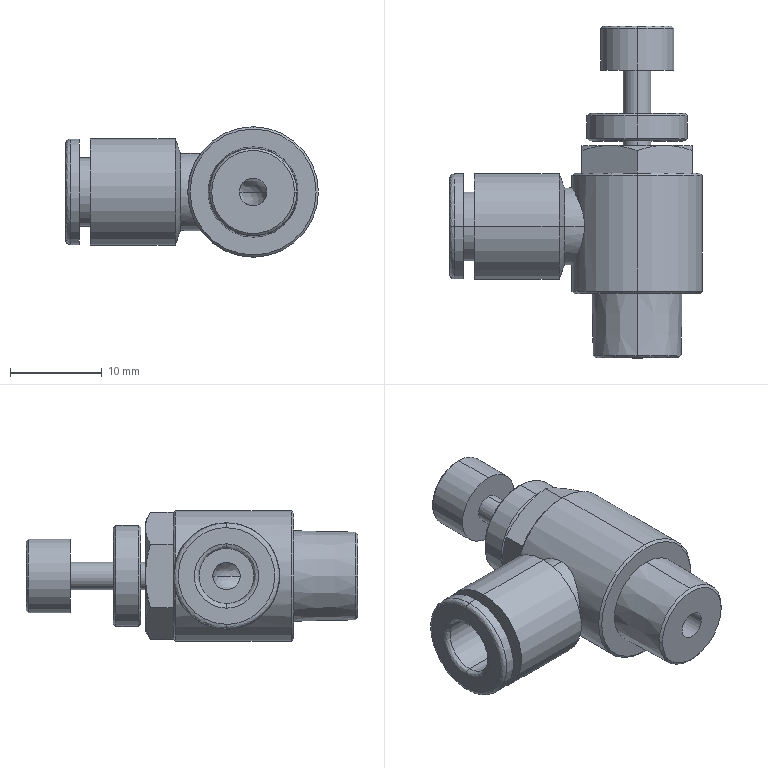Part | STEP file | Flow limiter AS2201F-01-06_SMC_22-01-06 | 1 solid | 82 faces | box 27.5 x 36.1 x 14.2 mm | volume 4282 mm3 | plane 29 | cylinder 24 | cone 23 | spline 6 | commonest cylinder face diameters 3 x8 6 x2 7.5 x2 8 x2 8.4 x2 11 x2